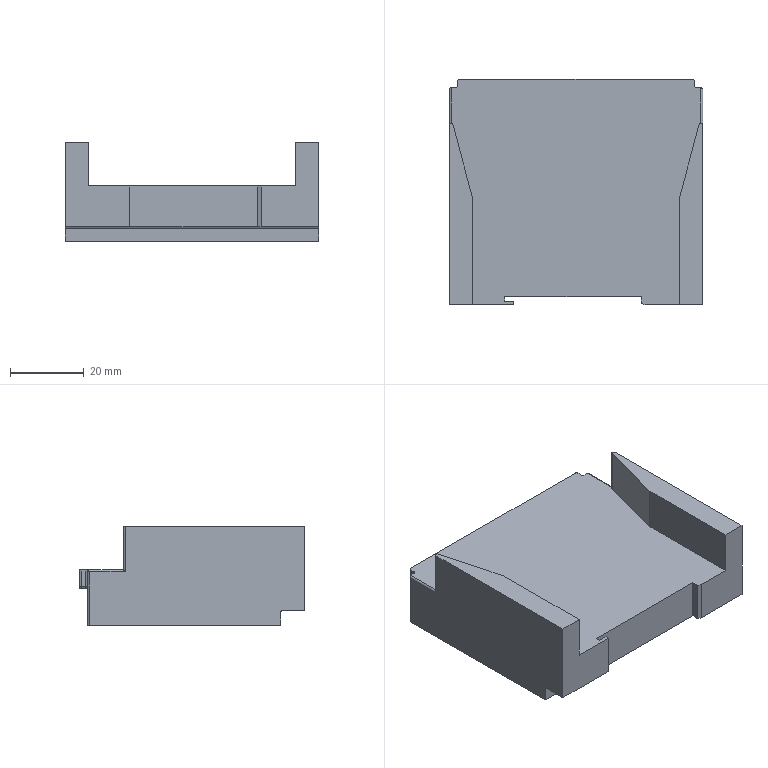Part | STEP file | SS5V1-16S3AD-08B-N1_EX120 Adapter | 1 solid | 46 faces | box 68.5 x 61 x 26.75 mm | volume 64315 mm3 | plane 25 | cylinder 17 | sphere 2 | torus 2 | commonest cylinder face diameters 1 x17